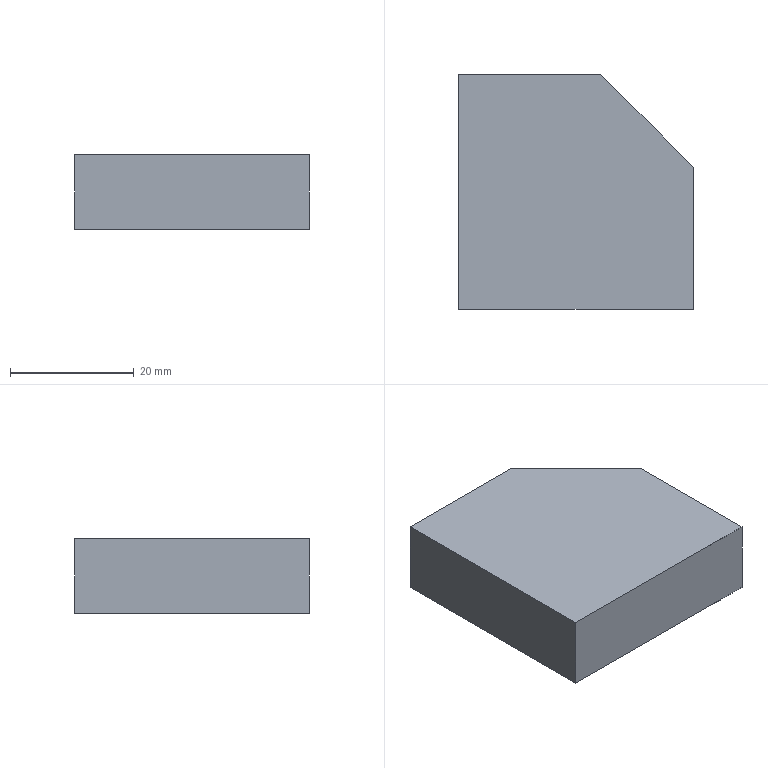Part | STEP file | [03]-2 | 1 solid | 7 faces | box 38 x 38 x 12 mm | volume 15978 mm3 | plane 7
STEP:
#1=CARTESIAN_POINT('',(38.,23.,12.));
#2=VERTEX_POINT('',#1);
#3=CARTESIAN_POINT('',(38.,0.,12.));
#4=VERTEX_POINT('',#3);
#5=CARTESIAN_POINT('',(38.,19.,12.));
#6=DIRECTION('',(0.,-1.,0.));
#7=VECTOR('',#6,1000.);
#8=LINE('',#5,#7);
#9=EDGE_CURVE('',#2,#4,#8,.T.);
#10=ORIENTED_EDGE('',*,*,#9,.F.);
#11=CARTESIAN_POINT('',(23.,38.,12.));
#12=VERTEX_POINT('',#11);
#13=CARTESIAN_POINT('',(30.5,30.5,12.));
#14=DIRECTION('',(-0.7071,0.7071,0.));
#15=VECTOR('',#14,1000.);
#16=LINE('',#13,#15);
#17=EDGE_CURVE('',#2,#12,#16,.T.);
#18=ORIENTED_EDGE('',*,*,#17,.T.);
#19=CARTESIAN_POINT('',(0.,38.,12.));
#20=VERTEX_POINT('',#19);
#21=CARTESIAN_POINT('',(19.,38.,12.));
#22=DIRECTION('',(1.,0.,0.));
#23=VECTOR('',#22,1000.);
#24=LINE('',#21,#23);
#25=EDGE_CURVE('',#20,#12,#24,.T.);
#26=ORIENTED_EDGE('',*,*,#25,.F.);
#27=CARTESIAN_POINT('',(0.,0.,12.));
#28=VERTEX_POINT('',#27);
#29=CARTESIAN_POINT('',(0.,19.,12.));
#30=DIRECTION('',(0.,1.,0.));
#31=VECTOR('',#30,1000.);
#32=LINE('',#29,#31);
#33=EDGE_CURVE('',#28,#20,#32,.T.);
#34=ORIENTED_EDGE('',*,*,#33,.F.);
#35=CARTESIAN_POINT('',(19.,0.,12.));
#36=DIRECTION('',(-1.,0.,0.));
#37=VECTOR('',#36,1000.);
#38=LINE('',#35,#37);
#39=EDGE_CURVE('',#4,#28,#38,.T.);
#40=ORIENTED_EDGE('',*,*,#39,.F.);
#41=EDGE_LOOP('',(#10,#18,#26,#34,#40));
#42=FACE_OUTER_BOUND('',#41,.T.);
#43=CARTESIAN_POINT('',(19.,19.,12.));
#44=DIRECTION('',(0.,0.,1.));
#45=DIRECTION('',(0.,1.,0.));
#46=AXIS2_PLACEMENT_3D('',#43,#44,#45);
#47=PLANE('',#46);
#48=ADVANCED_FACE('',(#42),#47,.T.);
#49=CARTESIAN_POINT('',(38.,0.,0.));
#50=VERTEX_POINT('',#49);
#51=CARTESIAN_POINT('',(38.,23.,0.));
#52=VERTEX_POINT('',#51);
#53=CARTESIAN_POINT('',(38.,19.,0.));
#54=DIRECTION('',(0.,1.,0.));
#55=VECTOR('',#54,1000.);
#56=LINE('',#53,#55);
#57=EDGE_CURVE('',#50,#52,#56,.T.);
#58=ORIENTED_EDGE('',*,*,#57,.T.);
#59=CARTESIAN_POINT('',(38.,23.,0.));
#60=DIRECTION('',(0.,0.,1.));
#61=VECTOR('',#60,1000.);
#62=LINE('',#59,#61);
#63=EDGE_CURVE('',#52,#2,#62,.T.);
#64=ORIENTED_EDGE('',*,*,#63,.T.);
#65=ORIENTED_EDGE('',*,*,#9,.T.);
#66=CARTESIAN_POINT('',(38.,0.,0.));
#67=DIRECTION('',(0.,0.,1.));
#68=VECTOR('',#67,1000.);
#69=LINE('',#66,#68);
#70=EDGE_CURVE('',#50,#4,#69,.T.);
#71=ORIENTED_EDGE('',*,*,#70,.F.);
#72=EDGE_LOOP('',(#58,#64,#65,#71));
#73=FACE_OUTER_BOUND('',#72,.T.);
#74=CARTESIAN_POINT('',(38.,19.,0.));
#75=DIRECTION('',(1.,0.,0.));
#76=DIRECTION('',(0.,0.,-1.));
#77=AXIS2_PLACEMENT_3D('',#74,#75,#76);
#78=PLANE('',#77);
#79=ADVANCED_FACE('',(#73),#78,.T.);
#80=ORIENTED_EDGE('',*,*,#70,.T.);
#81=ORIENTED_EDGE('',*,*,#39,.T.);
#82=CARTESIAN_POINT('',(0.,0.,0.));
#83=VERTEX_POINT('',#82);
#84=CARTESIAN_POINT('',(0.,0.,0.));
#85=DIRECTION('',(0.,0.,1.));
#86=VECTOR('',#85,1000.);
#87=LINE('',#84,#86);
#88=EDGE_CURVE('',#83,#28,#87,.T.);
#89=ORIENTED_EDGE('',*,*,#88,.F.);
#90=CARTESIAN_POINT('',(19.,0.,0.));
#91=DIRECTION('',(1.,0.,0.));
#92=VECTOR('',#91,1000.);
#93=LINE('',#90,#92);
#94=EDGE_CURVE('',#83,#50,#93,.T.);
#95=ORIENTED_EDGE('',*,*,#94,.T.);
#96=EDGE_LOOP('',(#80,#81,#89,#95));
#97=FACE_OUTER_BOUND('',#96,.T.);
#98=CARTESIAN_POINT('',(19.,0.,0.));
#99=DIRECTION('',(0.,-1.,0.));
#100=DIRECTION('',(0.,0.,1.));
#101=AXIS2_PLACEMENT_3D('',#98,#99,#100);
#102=PLANE('',#101);
#103=ADVANCED_FACE('',(#97),#102,.T.);
#104=ORIENTED_EDGE('',*,*,#88,.T.);
#105=ORIENTED_EDGE('',*,*,#33,.T.);
#106=CARTESIAN_POINT('',(0.,38.,0.));
#107=VERTEX_POINT('',#106);
#108=CARTESIAN_POINT('',(0.,38.,0.));
#109=DIRECTION('',(0.,0.,1.));
#110=VECTOR('',#109,1000.);
#111=LINE('',#108,#110);
#112=EDGE_CURVE('',#107,#20,#111,.T.);
#113=ORIENTED_EDGE('',*,*,#112,.F.);
#114=CARTESIAN_POINT('',(0.,19.,0.));
#115=DIRECTION('',(0.,-1.,0.));
#116=VECTOR('',#115,1000.);
#117=LINE('',#114,#116);
#118=EDGE_CURVE('',#107,#83,#117,.T.);
#119=ORIENTED_EDGE('',*,*,#118,.T.);
#120=EDGE_LOOP('',(#104,#105,#113,#119));
#121=FACE_OUTER_BOUND('',#120,.T.);
#122=CARTESIAN_POINT('',(0.,19.,0.));
#123=DIRECTION('',(-1.,0.,0.));
#124=DIRECTION('',(0.,0.,1.));
#125=AXIS2_PLACEMENT_3D('',#122,#123,#124);
#126=PLANE('',#125);
#127=ADVANCED_FACE('',(#121),#126,.T.);
#128=CARTESIAN_POINT('',(23.,38.,0.));
#129=VERTEX_POINT('',#128);
#130=CARTESIAN_POINT('',(19.,38.,0.));
#131=DIRECTION('',(-1.,0.,0.));
#132=VECTOR('',#131,1000.);
#133=LINE('',#130,#132);
#134=EDGE_CURVE('',#129,#107,#133,.T.);
#135=ORIENTED_EDGE('',*,*,#134,.F.);
#136=CARTESIAN_POINT('',(30.5,30.5,0.));
#137=DIRECTION('',(0.7071,-0.7071,0.));
#138=VECTOR('',#137,1000.);
#139=LINE('',#136,#138);
#140=EDGE_CURVE('',#129,#52,#139,.T.);
#141=ORIENTED_EDGE('',*,*,#140,.T.);
#142=ORIENTED_EDGE('',*,*,#57,.F.);
#143=ORIENTED_EDGE('',*,*,#94,.F.);
#144=ORIENTED_EDGE('',*,*,#118,.F.);
#145=EDGE_LOOP('',(#135,#141,#142,#143,#144));
#146=FACE_OUTER_BOUND('',#145,.T.);
#147=CARTESIAN_POINT('',(19.,19.,0.));
#148=DIRECTION('',(0.,0.,-1.));
#149=DIRECTION('',(0.,-1.,0.));
#150=AXIS2_PLACEMENT_3D('',#147,#148,#149);
#151=PLANE('',#150);
#152=ADVANCED_FACE('',(#146),#151,.T.);
#153=ORIENTED_EDGE('',*,*,#25,.T.);
#154=CARTESIAN_POINT('',(23.,38.,0.));
#155=DIRECTION('',(0.,0.,-1.));
#156=VECTOR('',#155,1000.);
#157=LINE('',#154,#156);
#158=EDGE_CURVE('',#12,#129,#157,.T.);
#159=ORIENTED_EDGE('',*,*,#158,.T.);
#160=ORIENTED_EDGE('',*,*,#134,.T.);
#161=ORIENTED_EDGE('',*,*,#112,.T.);
#162=EDGE_LOOP('',(#153,#159,#160,#161));
#163=FACE_OUTER_BOUND('',#162,.T.);
#164=CARTESIAN_POINT('',(19.,38.,0.));
#165=DIRECTION('',(0.,1.,0.));
#166=DIRECTION('',(0.,0.,-1.));
#167=AXIS2_PLACEMENT_3D('',#164,#165,#166);
#168=PLANE('',#167);
#169=ADVANCED_FACE('',(#163),#168,.T.);
#170=ORIENTED_EDGE('',*,*,#140,.F.);
#171=ORIENTED_EDGE('',*,*,#158,.F.);
#172=ORIENTED_EDGE('',*,*,#17,.F.);
#173=ORIENTED_EDGE('',*,*,#63,.F.);
#174=EDGE_LOOP('',(#170,#171,#172,#173));
#175=FACE_OUTER_BOUND('',#174,.T.);
#176=CARTESIAN_POINT('',(38.,23.,0.));
#177=DIRECTION('',(-0.7071,-0.7071,0.));
#178=DIRECTION('',(0.,0.,1.));
#179=AXIS2_PLACEMENT_3D('',#176,#177,#178);
#180=PLANE('',#179);
#181=ADVANCED_FACE('',(#175),#180,.F.);
#182=CLOSED_SHELL('',(#48,#79,#103,#127,#152,#169,#181));
#183=MANIFOLD_SOLID_BREP('',#182);
#184=CARTESIAN_POINT('',(0.,0.,0.));
#185=DIRECTION('',(0.,0.,1.));
#186=DIRECTION('',(1.,0.,0.));
#187=AXIS2_PLACEMENT_3D('',#184,#185,#186);
#188=(LENGTH_UNIT()NAMED_UNIT(*)SI_UNIT(.MILLI.,.METRE.));
#189=UNCERTAINTY_MEASURE_WITH_UNIT(LENGTH_MEASURE(0.00001),#188,'','');
#190=(NAMED_UNIT(*)PLANE_ANGLE_UNIT()SI_UNIT($,.RADIAN.));
#191=(NAMED_UNIT(*)SI_UNIT($,.STERADIAN.)SOLID_ANGLE_UNIT());
#192=(GEOMETRIC_REPRESENTATION_CONTEXT(3)GLOBAL_UNCERTAINTY_ASSIGNED_CONTEXT((#189))GLOBAL_UNIT_ASSIGNED_CONTEXT((#188,#190,#191))REPRESENTATION_CONTEXT('',''));
#193=ADVANCED_BREP_SHAPE_REPRESENTATION('',(#183,#187),#192);